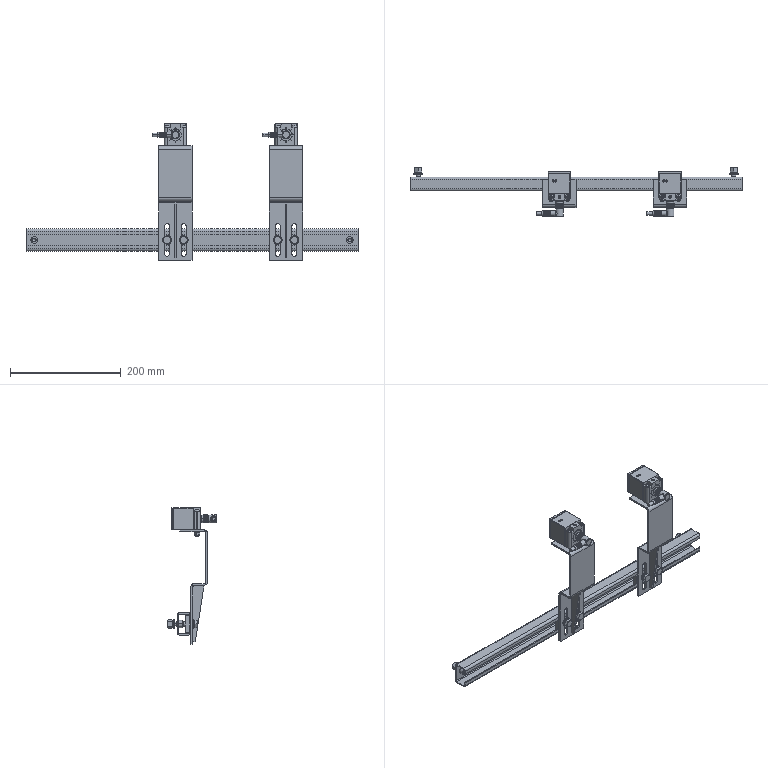Part | SolidWorks | 31 solids | 4372 faces | volume 438614 mm3 | spline 2448 | cylinder 936 | plane 798 | cone 190 | commonest cylinder face diameters 14.5 x550 2 x28 8 x28 9 x28 6 x26 1 x20